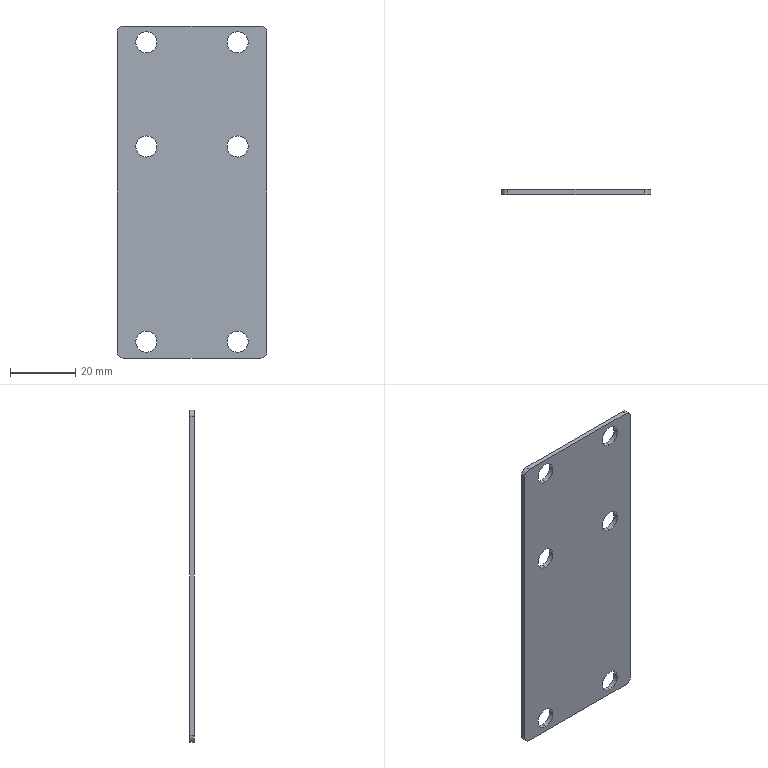Part | SolidWorks | features BaseBody 1 | 1 solid | 22 faces | box 46 x 1.5 x 102 mm | volume 6734 mm3 | cylinder 16 | plane 6 | commonest cylinder face diameters 6.5 x12 4 x4
STEP:
#1=CARTESIAN_POINT('',(14.,0.,-42.75));
#2=VERTEX_POINT('',#1);
#3=CARTESIAN_POINT('',(14.,0.,-49.25));
#4=VERTEX_POINT('',#3);
#5=CARTESIAN_POINT('',(14.,0.,-46.));
#6=DIRECTION('',(0.,1.,0.));
#7=DIRECTION('',(0.,0.,1.));
#8=AXIS2_PLACEMENT_3D('',#5,#6,#7);
#9=CIRCLE('',#8,3.25);
#10=EDGE_CURVE('',#2,#4,#9,.T.);
#11=ORIENTED_EDGE('',*,*,#10,.T.);
#12=CARTESIAN_POINT('',(14.,0.,-46.));
#13=DIRECTION('',(0.,1.,0.));
#14=DIRECTION('',(0.,0.,1.));
#15=AXIS2_PLACEMENT_3D('',#12,#13,#14);
#16=CIRCLE('',#15,3.25);
#17=EDGE_CURVE('',#4,#2,#16,.T.);
#18=ORIENTED_EDGE('',*,*,#17,.T.);
#19=EDGE_LOOP('',(#11,#18));
#20=FACE_BOUND('',#19,.T.);
#21=CARTESIAN_POINT('',(-14.,0.,-42.75));
#22=VERTEX_POINT('',#21);
#23=CARTESIAN_POINT('',(-14.,0.,-49.25));
#24=VERTEX_POINT('',#23);
#25=CARTESIAN_POINT('',(-14.,0.,-46.));
#26=DIRECTION('',(0.,1.,0.));
#27=DIRECTION('',(0.,0.,1.));
#28=AXIS2_PLACEMENT_3D('',#25,#26,#27);
#29=CIRCLE('',#28,3.25);
#30=EDGE_CURVE('',#22,#24,#29,.T.);
#31=ORIENTED_EDGE('',*,*,#30,.T.);
#32=CARTESIAN_POINT('',(-14.,0.,-46.));
#33=DIRECTION('',(0.,1.,0.));
#34=DIRECTION('',(0.,0.,1.));
#35=AXIS2_PLACEMENT_3D('',#32,#33,#34);
#36=CIRCLE('',#35,3.25);
#37=EDGE_CURVE('',#24,#22,#36,.T.);
#38=ORIENTED_EDGE('',*,*,#37,.T.);
#39=EDGE_LOOP('',(#31,#38));
#40=FACE_BOUND('',#39,.T.);
#41=CARTESIAN_POINT('',(-14.,0.,17.25));
#42=VERTEX_POINT('',#41);
#43=CARTESIAN_POINT('',(-14.,0.,10.75));
#44=VERTEX_POINT('',#43);
#45=CARTESIAN_POINT('',(-14.,0.,14.));
#46=DIRECTION('',(0.,1.,0.));
#47=DIRECTION('',(0.,0.,1.));
#48=AXIS2_PLACEMENT_3D('',#45,#46,#47);
#49=CIRCLE('',#48,3.25);
#50=EDGE_CURVE('',#42,#44,#49,.T.);
#51=ORIENTED_EDGE('',*,*,#50,.T.);
#52=CARTESIAN_POINT('',(-14.,0.,14.));
#53=DIRECTION('',(0.,1.,0.));
#54=DIRECTION('',(0.,0.,1.));
#55=AXIS2_PLACEMENT_3D('',#52,#53,#54);
#56=CIRCLE('',#55,3.25);
#57=EDGE_CURVE('',#44,#42,#56,.T.);
#58=ORIENTED_EDGE('',*,*,#57,.T.);
#59=EDGE_LOOP('',(#51,#58));
#60=FACE_BOUND('',#59,.T.);
#61=CARTESIAN_POINT('',(14.,0.,17.25));
#62=VERTEX_POINT('',#61);
#63=CARTESIAN_POINT('',(14.,0.,10.75));
#64=VERTEX_POINT('',#63);
#65=CARTESIAN_POINT('',(14.,0.,14.));
#66=DIRECTION('',(0.,1.,0.));
#67=DIRECTION('',(0.,0.,1.));
#68=AXIS2_PLACEMENT_3D('',#65,#66,#67);
#69=CIRCLE('',#68,3.25);
#70=EDGE_CURVE('',#62,#64,#69,.T.);
#71=ORIENTED_EDGE('',*,*,#70,.T.);
#72=CARTESIAN_POINT('',(14.,0.,14.));
#73=DIRECTION('',(0.,1.,0.));
#74=DIRECTION('',(0.,0.,1.));
#75=AXIS2_PLACEMENT_3D('',#72,#73,#74);
#76=CIRCLE('',#75,3.25);
#77=EDGE_CURVE('',#64,#62,#76,.T.);
#78=ORIENTED_EDGE('',*,*,#77,.T.);
#79=EDGE_LOOP('',(#71,#78));
#80=FACE_BOUND('',#79,.T.);
#81=CARTESIAN_POINT('',(-14.,0.,49.25));
#82=VERTEX_POINT('',#81);
#83=CARTESIAN_POINT('',(-14.,0.,42.75));
#84=VERTEX_POINT('',#83);
#85=CARTESIAN_POINT('',(-14.,0.,46.));
#86=DIRECTION('',(0.,1.,0.));
#87=DIRECTION('',(0.,0.,1.));
#88=AXIS2_PLACEMENT_3D('',#85,#86,#87);
#89=CIRCLE('',#88,3.25);
#90=EDGE_CURVE('',#82,#84,#89,.T.);
#91=ORIENTED_EDGE('',*,*,#90,.T.);
#92=CARTESIAN_POINT('',(-14.,0.,46.));
#93=DIRECTION('',(0.,1.,0.));
#94=DIRECTION('',(0.,0.,1.));
#95=AXIS2_PLACEMENT_3D('',#92,#93,#94);
#96=CIRCLE('',#95,3.25);
#97=EDGE_CURVE('',#84,#82,#96,.T.);
#98=ORIENTED_EDGE('',*,*,#97,.T.);
#99=EDGE_LOOP('',(#91,#98));
#100=FACE_BOUND('',#99,.T.);
#101=CARTESIAN_POINT('',(14.,0.,49.25));
#102=VERTEX_POINT('',#101);
#103=CARTESIAN_POINT('',(14.,0.,42.75));
#104=VERTEX_POINT('',#103);
#105=CARTESIAN_POINT('',(14.,0.,46.));
#106=DIRECTION('',(0.,1.,0.));
#107=DIRECTION('',(0.,0.,1.));
#108=AXIS2_PLACEMENT_3D('',#105,#106,#107);
#109=CIRCLE('',#108,3.25);
#110=EDGE_CURVE('',#102,#104,#109,.T.);
#111=ORIENTED_EDGE('',*,*,#110,.T.);
#112=CARTESIAN_POINT('',(14.,0.,46.));
#113=DIRECTION('',(0.,1.,0.));
#114=DIRECTION('',(0.,0.,1.));
#115=AXIS2_PLACEMENT_3D('',#112,#113,#114);
#116=CIRCLE('',#115,3.25);
#117=EDGE_CURVE('',#104,#102,#116,.T.);
#118=ORIENTED_EDGE('',*,*,#117,.T.);
#119=EDGE_LOOP('',(#111,#118));
#120=FACE_BOUND('',#119,.T.);
#121=CARTESIAN_POINT('',(-23.,0.,49.));
#122=VERTEX_POINT('',#121);
#123=CARTESIAN_POINT('',(-23.,0.,-49.));
#124=VERTEX_POINT('',#123);
#125=CARTESIAN_POINT('',(-23.,0.,-51.));
#126=DIRECTION('',(0.,0.,-1.));
#127=VECTOR('',#126,1000.);
#128=LINE('',#125,#127);
#129=EDGE_CURVE('',#122,#124,#128,.T.);
#130=ORIENTED_EDGE('',*,*,#129,.T.);
#131=CARTESIAN_POINT('',(-21.,0.,-51.));
#132=VERTEX_POINT('',#131);
#133=CARTESIAN_POINT('',(-21.,0.,-49.));
#134=DIRECTION('',(0.,1.,0.));
#135=DIRECTION('',(0.,0.,-1.));
#136=AXIS2_PLACEMENT_3D('',#133,#134,#135);
#137=CIRCLE('',#136,2.);
#138=EDGE_CURVE('',#132,#124,#137,.T.);
#139=ORIENTED_EDGE('',*,*,#138,.F.);
#140=CARTESIAN_POINT('',(21.,0.,-51.));
#141=VERTEX_POINT('',#140);
#142=CARTESIAN_POINT('',(-23.,0.,-51.));
#143=DIRECTION('',(1.,0.,0.));
#144=VECTOR('',#143,1000.);
#145=LINE('',#142,#144);
#146=EDGE_CURVE('',#132,#141,#145,.T.);
#147=ORIENTED_EDGE('',*,*,#146,.T.);
#148=CARTESIAN_POINT('',(23.,0.,-49.));
#149=VERTEX_POINT('',#148);
#150=CARTESIAN_POINT('',(21.,0.,-49.));
#151=DIRECTION('',(0.,1.,0.));
#152=DIRECTION('',(0.,0.,-1.));
#153=AXIS2_PLACEMENT_3D('',#150,#151,#152);
#154=CIRCLE('',#153,2.);
#155=EDGE_CURVE('',#149,#141,#154,.T.);
#156=ORIENTED_EDGE('',*,*,#155,.F.);
#157=CARTESIAN_POINT('',(23.,0.,49.));
#158=VERTEX_POINT('',#157);
#159=CARTESIAN_POINT('',(23.,0.,-51.));
#160=DIRECTION('',(0.,0.,1.));
#161=VECTOR('',#160,1000.);
#162=LINE('',#159,#161);
#163=EDGE_CURVE('',#149,#158,#162,.T.);
#164=ORIENTED_EDGE('',*,*,#163,.T.);
#165=CARTESIAN_POINT('',(21.,0.,51.));
#166=VERTEX_POINT('',#165);
#167=CARTESIAN_POINT('',(21.,0.,49.));
#168=DIRECTION('',(0.,1.,0.));
#169=DIRECTION('',(0.,0.,-1.));
#170=AXIS2_PLACEMENT_3D('',#167,#168,#169);
#171=CIRCLE('',#170,2.);
#172=EDGE_CURVE('',#166,#158,#171,.T.);
#173=ORIENTED_EDGE('',*,*,#172,.F.);
#174=CARTESIAN_POINT('',(-21.,0.,51.));
#175=VERTEX_POINT('',#174);
#176=CARTESIAN_POINT('',(-23.,0.,51.));
#177=DIRECTION('',(-1.,0.,0.));
#178=VECTOR('',#177,1000.);
#179=LINE('',#176,#178);
#180=EDGE_CURVE('',#166,#175,#179,.T.);
#181=ORIENTED_EDGE('',*,*,#180,.T.);
#182=CARTESIAN_POINT('',(-21.,0.,49.));
#183=DIRECTION('',(0.,1.,0.));
#184=DIRECTION('',(0.,0.,-1.));
#185=AXIS2_PLACEMENT_3D('',#182,#183,#184);
#186=CIRCLE('',#185,2.);
#187=EDGE_CURVE('',#122,#175,#186,.T.);
#188=ORIENTED_EDGE('',*,*,#187,.F.);
#189=EDGE_LOOP('',(#130,#139,#147,#156,#164,#173,#181,#188));
#190=FACE_OUTER_BOUND('',#189,.T.);
#191=CARTESIAN_POINT('',(0.,0.,0.));
#192=DIRECTION('',(0.,1.,0.));
#193=DIRECTION('',(1.,0.,0.));
#194=AXIS2_PLACEMENT_3D('',#191,#192,#193);
#195=PLANE('',#194);
#196=ADVANCED_FACE('',(#20,#40,#60,#80,#100,#120,#190),#195,.F.);
#197=ORIENTED_EDGE('',*,*,#146,.F.);
#198=CARTESIAN_POINT('',(-21.,1.5,-51.));
#199=VERTEX_POINT('',#198);
#200=CARTESIAN_POINT('',(-21.,1.5,-51.));
#201=DIRECTION('',(0.,-1.,0.));
#202=VECTOR('',#201,1000.);
#203=LINE('',#200,#202);
#204=EDGE_CURVE('',#199,#132,#203,.T.);
#205=ORIENTED_EDGE('',*,*,#204,.F.);
#206=CARTESIAN_POINT('',(21.,1.5,-51.));
#207=VERTEX_POINT('',#206);
#208=CARTESIAN_POINT('',(0.,1.5,-51.));
#209=DIRECTION('',(-1.,0.,0.));
#210=VECTOR('',#209,1000.);
#211=LINE('',#208,#210);
#212=EDGE_CURVE('',#207,#199,#211,.T.);
#213=ORIENTED_EDGE('',*,*,#212,.F.);
#214=CARTESIAN_POINT('',(21.,1.5,-51.));
#215=DIRECTION('',(0.,1.,0.));
#216=VECTOR('',#215,1000.);
#217=LINE('',#214,#216);
#218=EDGE_CURVE('',#141,#207,#217,.T.);
#219=ORIENTED_EDGE('',*,*,#218,.F.);
#220=EDGE_LOOP('',(#197,#205,#213,#219));
#221=FACE_OUTER_BOUND('',#220,.T.);
#222=CARTESIAN_POINT('',(-23.,1.5,-51.));
#223=DIRECTION('',(0.,0.,1.));
#224=DIRECTION('',(1.,0.,0.));
#225=AXIS2_PLACEMENT_3D('',#222,#223,#224);
#226=PLANE('',#225);
#227=ADVANCED_FACE('',(#221),#226,.F.);
#228=CARTESIAN_POINT('',(-23.,1.5,-49.));
#229=VERTEX_POINT('',#228);
#230=CARTESIAN_POINT('',(-21.,1.5,-49.));
#231=DIRECTION('',(0.,1.,0.));
#232=DIRECTION('',(0.,0.,-1.));
#233=AXIS2_PLACEMENT_3D('',#230,#231,#232);
#234=CIRCLE('',#233,2.);
#235=EDGE_CURVE('',#199,#229,#234,.T.);
#236=ORIENTED_EDGE('',*,*,#235,.F.);
#237=ORIENTED_EDGE('',*,*,#204,.T.);
#238=ORIENTED_EDGE('',*,*,#138,.T.);
#239=CARTESIAN_POINT('',(-23.,1.5,-49.));
#240=DIRECTION('',(0.,1.,0.));
#241=VECTOR('',#240,1000.);
#242=LINE('',#239,#241);
#243=EDGE_CURVE('',#124,#229,#242,.T.);
#244=ORIENTED_EDGE('',*,*,#243,.T.);
#245=EDGE_LOOP('',(#236,#237,#238,#244));
#246=FACE_OUTER_BOUND('',#245,.T.);
#247=CARTESIAN_POINT('',(-21.,1.5,-49.));
#248=DIRECTION('',(0.,-1.,0.));
#249=DIRECTION('',(0.,0.,-1.));
#250=AXIS2_PLACEMENT_3D('',#247,#248,#249);
#251=CYLINDRICAL_SURFACE('',#250,2.);
#252=ADVANCED_FACE('',(#246),#251,.T.);
#253=CARTESIAN_POINT('',(-23.,1.5,49.));
#254=VERTEX_POINT('',#253);
#255=CARTESIAN_POINT('',(-23.,1.5,0.));
#256=DIRECTION('',(0.,0.,1.));
#257=VECTOR('',#256,1000.);
#258=LINE('',#255,#257);
#259=EDGE_CURVE('',#229,#254,#258,.T.);
#260=ORIENTED_EDGE('',*,*,#259,.F.);
#261=ORIENTED_EDGE('',*,*,#243,.F.);
#262=ORIENTED_EDGE('',*,*,#129,.F.);
#263=CARTESIAN_POINT('',(-23.,1.5,49.));
#264=DIRECTION('',(0.,-1.,0.));
#265=VECTOR('',#264,1000.);
#266=LINE('',#263,#265);
#267=EDGE_CURVE('',#254,#122,#266,.T.);
#268=ORIENTED_EDGE('',*,*,#267,.F.);
#269=EDGE_LOOP('',(#260,#261,#262,#268));
#270=FACE_OUTER_BOUND('',#269,.T.);
#271=CARTESIAN_POINT('',(-23.,1.5,-51.));
#272=DIRECTION('',(1.,0.,0.));
#273=DIRECTION('',(0.,0.,-1.));
#274=AXIS2_PLACEMENT_3D('',#271,#272,#273);
#275=PLANE('',#274);
#276=ADVANCED_FACE('',(#270),#275,.F.);
#277=CARTESIAN_POINT('',(-21.,1.5,51.));
#278=VERTEX_POINT('',#277);
#279=CARTESIAN_POINT('',(-21.,1.5,49.));
#280=DIRECTION('',(0.,1.,0.));
#281=DIRECTION('',(0.,0.,-1.));
#282=AXIS2_PLACEMENT_3D('',#279,#280,#281);
#283=CIRCLE('',#282,2.);
#284=EDGE_CURVE('',#254,#278,#283,.T.);
#285=ORIENTED_EDGE('',*,*,#284,.F.);
#286=ORIENTED_EDGE('',*,*,#267,.T.);
#287=ORIENTED_EDGE('',*,*,#187,.T.);
#288=CARTESIAN_POINT('',(-21.,1.5,51.));
#289=DIRECTION('',(0.,1.,0.));
#290=VECTOR('',#289,1000.);
#291=LINE('',#288,#290);
#292=EDGE_CURVE('',#175,#278,#291,.T.);
#293=ORIENTED_EDGE('',*,*,#292,.T.);
#294=EDGE_LOOP('',(#285,#286,#287,#293));
#295=FACE_OUTER_BOUND('',#294,.T.);
#296=CARTESIAN_POINT('',(-21.,1.5,49.));
#297=DIRECTION('',(0.,-1.,0.));
#298=DIRECTION('',(0.,0.,-1.));
#299=AXIS2_PLACEMENT_3D('',#296,#297,#298);
#300=CYLINDRICAL_SURFACE('',#299,2.);
#301=ADVANCED_FACE('',(#295),#300,.T.);
#302=ORIENTED_EDGE('',*,*,#180,.F.);
#303=CARTESIAN_POINT('',(21.,1.5,51.));
#304=VERTEX_POINT('',#303);
#305=CARTESIAN_POINT('',(21.,1.5,51.));
#306=DIRECTION('',(0.,-1.,0.));
#307=VECTOR('',#306,1000.);
#308=LINE('',#305,#307);
#309=EDGE_CURVE('',#304,#166,#308,.T.);
#310=ORIENTED_EDGE('',*,*,#309,.F.);
#311=CARTESIAN_POINT('',(0.,1.5,51.));
#312=DIRECTION('',(1.,0.,0.));
#313=VECTOR('',#312,1000.);
#314=LINE('',#311,#313);
#315=EDGE_CURVE('',#278,#304,#314,.T.);
#316=ORIENTED_EDGE('',*,*,#315,.F.);
#317=ORIENTED_EDGE('',*,*,#292,.F.);
#318=EDGE_LOOP('',(#302,#310,#316,#317));
#319=FACE_OUTER_BOUND('',#318,.T.);
#320=CARTESIAN_POINT('',(-23.,1.5,51.));
#321=DIRECTION('',(0.,0.,-1.));
#322=DIRECTION('',(0.,-1.,0.));
#323=AXIS2_PLACEMENT_3D('',#320,#321,#322);
#324=PLANE('',#323);
#325=ADVANCED_FACE('',(#319),#324,.F.);
#326=CARTESIAN_POINT('',(23.,1.5,49.));
#327=VERTEX_POINT('',#326);
#328=CARTESIAN_POINT('',(21.,1.5,49.));
#329=DIRECTION('',(0.,1.,0.));
#330=DIRECTION('',(0.,0.,-1.));
#331=AXIS2_PLACEMENT_3D('',#328,#329,#330);
#332=CIRCLE('',#331,2.);
#333=EDGE_CURVE('',#304,#327,#332,.T.);
#334=ORIENTED_EDGE('',*,*,#333,.F.);
#335=ORIENTED_EDGE('',*,*,#309,.T.);
#336=ORIENTED_EDGE('',*,*,#172,.T.);
#337=CARTESIAN_POINT('',(23.,1.5,49.));
#338=DIRECTION('',(0.,1.,0.));
#339=VECTOR('',#338,1000.);
#340=LINE('',#337,#339);
#341=EDGE_CURVE('',#158,#327,#340,.T.);
#342=ORIENTED_EDGE('',*,*,#341,.T.);
#343=EDGE_LOOP('',(#334,#335,#336,#342));
#344=FACE_OUTER_BOUND('',#343,.T.);
#345=CARTESIAN_POINT('',(21.,1.5,49.));
#346=DIRECTION('',(0.,-1.,0.));
#347=DIRECTION('',(0.,0.,-1.));
#348=AXIS2_PLACEMENT_3D('',#345,#346,#347);
#349=CYLINDRICAL_SURFACE('',#348,2.);
#350=ADVANCED_FACE('',(#344),#349,.T.);
#351=ORIENTED_EDGE('',*,*,#163,.F.);
#352=CARTESIAN_POINT('',(23.,1.5,-49.));
#353=VERTEX_POINT('',#352);
#354=CARTESIAN_POINT('',(23.,1.5,-49.));
#355=DIRECTION('',(0.,-1.,0.));
#356=VECTOR('',#355,1000.);
#357=LINE('',#354,#356);
#358=EDGE_CURVE('',#353,#149,#357,.T.);
#359=ORIENTED_EDGE('',*,*,#358,.F.);
#360=CARTESIAN_POINT('',(23.,1.5,0.));
#361=DIRECTION('',(0.,0.,-1.));
#362=VECTOR('',#361,1000.);
#363=LINE('',#360,#362);
#364=EDGE_CURVE('',#327,#353,#363,.T.);
#365=ORIENTED_EDGE('',*,*,#364,.F.);
#366=ORIENTED_EDGE('',*,*,#341,.F.);
#367=EDGE_LOOP('',(#351,#359,#365,#366));
#368=FACE_OUTER_BOUND('',#367,.T.);
#369=CARTESIAN_POINT('',(23.,1.5,-51.));
#370=DIRECTION('',(-1.,0.,0.));
#371=DIRECTION('',(0.,1.,0.));
#372=AXIS2_PLACEMENT_3D('',#369,#370,#371);
#373=PLANE('',#372);
#374=ADVANCED_FACE('',(#368),#373,.F.);
#375=CARTESIAN_POINT('',(21.,1.5,-49.));
#376=DIRECTION('',(0.,1.,0.));
#377=DIRECTION('',(0.,0.,-1.));
#378=AXIS2_PLACEMENT_3D('',#375,#376,#377);
#379=CIRCLE('',#378,2.);
#380=EDGE_CURVE('',#353,#207,#379,.T.);
#381=ORIENTED_EDGE('',*,*,#380,.F.);
#382=ORIENTED_EDGE('',*,*,#358,.T.);
#383=ORIENTED_EDGE('',*,*,#155,.T.);
#384=ORIENTED_EDGE('',*,*,#218,.T.);
#385=EDGE_LOOP('',(#381,#382,#383,#384));
#386=FACE_OUTER_BOUND('',#385,.T.);
#387=CARTESIAN_POINT('',(21.,1.5,-49.));
#388=DIRECTION('',(0.,-1.,0.));
#389=DIRECTION('',(0.,0.,-1.));
#390=AXIS2_PLACEMENT_3D('',#387,#388,#389);
#391=CYLINDRICAL_SURFACE('',#390,2.);
#392=ADVANCED_FACE('',(#386),#391,.T.);
#393=CARTESIAN_POINT('',(14.,1.5,-49.25));
#394=VERTEX_POINT('',#393);
#395=CARTESIAN_POINT('',(14.,1.5,-49.25));
#396=DIRECTION('',(0.,1.,0.));
#397=VECTOR('',#396,1000.);
#398=LINE('',#395,#397);
#399=EDGE_CURVE('',#4,#394,#398,.T.);
#400=ORIENTED_EDGE('',*,*,#399,.F.);
#401=ORIENTED_EDGE('',*,*,#10,.F.);
#402=CARTESIAN_POINT('',(14.,1.5,-42.75));
#403=VERTEX_POINT('',#402);
#404=CARTESIAN_POINT('',(14.,1.5,-42.75));
#405=DIRECTION('',(0.,1.,0.));
#406=VECTOR('',#405,1000.);
#407=LINE('',#404,#406);
#408=EDGE_CURVE('',#2,#403,#407,.T.);
#409=ORIENTED_EDGE('',*,*,#408,.T.);
#410=CARTESIAN_POINT('',(14.,1.5,-46.));
#411=DIRECTION('',(0.,-1.,0.));
#412=DIRECTION('',(0.,0.,1.));
#413=AXIS2_PLACEMENT_3D('',#410,#411,#412);
#414=CIRCLE('',#413,3.25);
#415=EDGE_CURVE('',#394,#403,#414,.T.);
#416=ORIENTED_EDGE('',*,*,#415,.F.);
#417=EDGE_LOOP('',(#400,#401,#409,#416));
#418=FACE_OUTER_BOUND('',#417,.T.);
#419=CARTESIAN_POINT('',(14.,1.5,-46.));
#420=DIRECTION('',(0.,1.,0.));
#421=DIRECTION('',(0.,0.,1.));
#422=AXIS2_PLACEMENT_3D('',#419,#420,#421);
#423=CYLINDRICAL_SURFACE('',#422,3.25);
#424=ADVANCED_FACE('',(#418),#423,.F.);
#425=CARTESIAN_POINT('',(-14.,1.5,-49.25));
#426=VERTEX_POINT('',#425);
#427=CARTESIAN_POINT('',(-14.,1.5,-49.25));
#428=DIRECTION('',(0.,1.,0.));
#429=VECTOR('',#428,1000.);
#430=LINE('',#427,#429);
#431=EDGE_CURVE('',#24,#426,#430,.T.);
#432=ORIENTED_EDGE('',*,*,#431,.F.);
#433=ORIENTED_EDGE('',*,*,#30,.F.);
#434=CARTESIAN_POINT('',(-14.,1.5,-42.75));
#435=VERTEX_POINT('',#434);
#436=CARTESIAN_POINT('',(-14.,1.5,-42.75));
#437=DIRECTION('',(0.,1.,0.));
#438=VECTOR('',#437,1000.);
#439=LINE('',#436,#438);
#440=EDGE_CURVE('',#22,#435,#439,.T.);
#441=ORIENTED_EDGE('',*,*,#440,.T.);
#442=CARTESIAN_POINT('',(-14.,1.5,-46.));
#443=DIRECTION('',(0.,-1.,0.));
#444=DIRECTION('',(0.,0.,1.));
#445=AXIS2_PLACEMENT_3D('',#442,#443,#444);
#446=CIRCLE('',#445,3.25);
#447=EDGE_CURVE('',#426,#435,#446,.T.);
#448=ORIENTED_EDGE('',*,*,#447,.F.);
#449=EDGE_LOOP('',(#432,#433,#441,#448));
#450=FACE_OUTER_BOUND('',#449,.T.);
#451=CARTESIAN_POINT('',(-14.,1.5,-46.));
#452=DIRECTION('',(0.,1.,0.));
#453=DIRECTION('',(0.,0.,1.));
#454=AXIS2_PLACEMENT_3D('',#451,#452,#453);
#455=CYLINDRICAL_SURFACE('',#454,3.25);
#456=ADVANCED_FACE('',(#450),#455,.F.);
#457=CARTESIAN_POINT('',(-14.,1.5,10.75));
#458=VERTEX_POINT('',#457);
#459=CARTESIAN_POINT('',(-14.,1.5,10.75));
#460=DIRECTION('',(0.,1.,0.));
#461=VECTOR('',#460,1000.);
#462=LINE('',#459,#461);
#463=EDGE_CURVE('',#44,#458,#462,.T.);
#464=ORIENTED_EDGE('',*,*,#463,.F.);
#465=ORIENTED_EDGE('',*,*,#50,.F.);
#466=CARTESIAN_POINT('',(-14.,1.5,17.25));
#467=VERTEX_POINT('',#466);
#468=CARTESIAN_POINT('',(-14.,1.5,17.25));
#469=DIRECTION('',(0.,1.,0.));
#470=VECTOR('',#469,1000.);
#471=LINE('',#468,#470);
#472=EDGE_CURVE('',#42,#467,#471,.T.);
#473=ORIENTED_EDGE('',*,*,#472,.T.);
#474=CARTESIAN_POINT('',(-14.,1.5,14.));
#475=DIRECTION('',(0.,-1.,0.));
#476=DIRECTION('',(0.,0.,1.));
#477=AXIS2_PLACEMENT_3D('',#474,#475,#476);
#478=CIRCLE('',#477,3.25);
#479=EDGE_CURVE('',#458,#467,#478,.T.);
#480=ORIENTED_EDGE('',*,*,#479,.F.);
#481=EDGE_LOOP('',(#464,#465,#473,#480));
#482=FACE_OUTER_BOUND('',#481,.T.);
#483=CARTESIAN_POINT('',(-14.,1.5,14.));
#484=DIRECTION('',(0.,1.,0.));
#485=DIRECTION('',(0.,0.,1.));
#486=AXIS2_PLACEMENT_3D('',#483,#484,#485);
#487=CYLINDRICAL_SURFACE('',#486,3.25);
#488=ADVANCED_FACE('',(#482),#487,.F.);
#489=CARTESIAN_POINT('',(14.,1.5,10.75));
#490=VERTEX_POINT('',#489);
#491=CARTESIAN_POINT('',(14.,1.5,10.75));
#492=DIRECTION('',(0.,1.,0.));
#493=VECTOR('',#492,1000.);
#494=LINE('',#491,#493);
#495=EDGE_CURVE('',#64,#490,#494,.T.);
#496=ORIENTED_EDGE('',*,*,#495,.F.);
#497=ORIENTED_EDGE('',*,*,#70,.F.);
#498=CARTESIAN_POINT('',(14.,1.5,17.25));
#499=VERTEX_POINT('',#498);
#500=CARTESIAN_POINT('',(14.,1.5,17.25));
#501=DIRECTION('',(0.,1.,0.));
#502=VECTOR('',#501,1000.);
#503=LINE('',#500,#502);
#504=EDGE_CURVE('',#62,#499,#503,.T.);
#505=ORIENTED_EDGE('',*,*,#504,.T.);
#506=CARTESIAN_POINT('',(14.,1.5,14.));
#507=DIRECTION('',(0.,-1.,0.));
#508=DIRECTION('',(0.,0.,1.));
#509=AXIS2_PLACEMENT_3D('',#506,#507,#508);
#510=CIRCLE('',#509,3.25);
#511=EDGE_CURVE('',#490,#499,#510,.T.);
#512=ORIENTED_EDGE('',*,*,#511,.F.);
#513=EDGE_LOOP('',(#496,#497,#505,#512));
#514=FACE_OUTER_BOUND('',#513,.T.);
#515=CARTESIAN_POINT('',(14.,1.5,14.));
#516=DIRECTION('',(0.,1.,0.));
#517=DIRECTION('',(0.,0.,1.));
#518=AXIS2_PLACEMENT_3D('',#515,#516,#517);
#519=CYLINDRICAL_SURFACE('',#518,3.25);
#520=ADVANCED_FACE('',(#514),#519,.F.);
#521=CARTESIAN_POINT('',(-14.,1.5,42.75));
#522=VERTEX_POINT('',#521);
#523=CARTESIAN_POINT('',(-14.,1.5,42.75));
#524=DIRECTION('',(0.,1.,0.));
#525=VECTOR('',#524,1000.);
#526=LINE('',#523,#525);
#527=EDGE_CURVE('',#84,#522,#526,.T.);
#528=ORIENTED_EDGE('',*,*,#527,.F.);
#529=ORIENTED_EDGE('',*,*,#90,.F.);
#530=CARTESIAN_POINT('',(-14.,1.5,49.25));
#531=VERTEX_POINT('',#530);
#532=CARTESIAN_POINT('',(-14.,1.5,49.25));
#533=DIRECTION('',(0.,1.,0.));
#534=VECTOR('',#533,1000.);
#535=LINE('',#532,#534);
#536=EDGE_CURVE('',#82,#531,#535,.T.);
#537=ORIENTED_EDGE('',*,*,#536,.T.);
#538=CARTESIAN_POINT('',(-14.,1.5,46.));
#539=DIRECTION('',(0.,-1.,0.));
#540=DIRECTION('',(0.,0.,1.));
#541=AXIS2_PLACEMENT_3D('',#538,#539,#540);
#542=CIRCLE('',#541,3.25);
#543=EDGE_CURVE('',#522,#531,#542,.T.);
#544=ORIENTED_EDGE('',*,*,#543,.F.);
#545=EDGE_LOOP('',(#528,#529,#537,#544));
#546=FACE_OUTER_BOUND('',#545,.T.);
#547=CARTESIAN_POINT('',(-14.,1.5,46.));
#548=DIRECTION('',(0.,1.,0.));
#549=DIRECTION('',(0.,0.,1.));
#550=AXIS2_PLACEMENT_3D('',#547,#548,#549);
#551=CYLINDRICAL_SURFACE('',#550,3.25);
#552=ADVANCED_FACE('',(#546),#551,.F.);
#553=CARTESIAN_POINT('',(14.,1.5,42.75));
#554=VERTEX_POINT('',#553);
#555=CARTESIAN_POINT('',(14.,1.5,42.75));
#556=DIRECTION('',(0.,1.,0.));
#557=VECTOR('',#556,1000.);
#558=LINE('',#555,#557);
#559=EDGE_CURVE('',#104,#554,#558,.T.);
#560=ORIENTED_EDGE('',*,*,#559,.F.);
#561=ORIENTED_EDGE('',*,*,#110,.F.);
#562=CARTESIAN_POINT('',(14.,1.5,49.25));
#563=VERTEX_POINT('',#562);
#564=CARTESIAN_POINT('',(14.,1.5,49.25));
#565=DIRECTION('',(0.,1.,0.));
#566=VECTOR('',#565,1000.);
#567=LINE('',#564,#566);
#568=EDGE_CURVE('',#102,#563,#567,.T.);
#569=ORIENTED_EDGE('',*,*,#568,.T.);
#570=CARTESIAN_POINT('',(14.,1.5,46.));
#571=DIRECTION('',(0.,-1.,0.));
#572=DIRECTION('',(0.,0.,1.));
#573=AXIS2_PLACEMENT_3D('',#570,#571,#572);
#574=CIRCLE('',#573,3.25);
#575=EDGE_CURVE('',#554,#563,#574,.T.);
#576=ORIENTED_EDGE('',*,*,#575,.F.);
#577=EDGE_LOOP('',(#560,#561,#569,#576));
#578=FACE_OUTER_BOUND('',#577,.T.);
#579=CARTESIAN_POINT('',(14.,1.5,46.));
#580=DIRECTION('',(0.,1.,0.));
#581=DIRECTION('',(0.,0.,1.));
#582=AXIS2_PLACEMENT_3D('',#579,#580,#581);
#583=CYLINDRICAL_SURFACE('',#582,3.25);
#584=ADVANCED_FACE('',(#578),#583,.F.);
#585=CARTESIAN_POINT('',(14.,1.5,-46.));
#586=DIRECTION('',(0.,-1.,0.));
#587=DIRECTION('',(0.,0.,1.));
#588=AXIS2_PLACEMENT_3D('',#585,#586,#587);
#589=CIRCLE('',#588,3.25);
#590=EDGE_CURVE('',#403,#394,#589,.T.);
#591=ORIENTED_EDGE('',*,*,#590,.T.);
#592=ORIENTED_EDGE('',*,*,#415,.T.);
#593=EDGE_LOOP('',(#591,#592));
#594=FACE_BOUND('',#593,.T.);
#595=CARTESIAN_POINT('',(-14.,1.5,-46.));
#596=DIRECTION('',(0.,-1.,0.));
#597=DIRECTION('',(0.,0.,1.));
#598=AXIS2_PLACEMENT_3D('',#595,#596,#597);
#599=CIRCLE('',#598,3.25);
#600=EDGE_CURVE('',#435,#426,#599,.T.);
#601=ORIENTED_EDGE('',*,*,#600,.T.);
#602=ORIENTED_EDGE('',*,*,#447,.T.);
#603=EDGE_LOOP('',(#601,#602));
#604=FACE_BOUND('',#603,.T.);
#605=CARTESIAN_POINT('',(-14.,1.5,14.));
#606=DIRECTION('',(0.,-1.,0.));
#607=DIRECTION('',(0.,0.,1.));
#608=AXIS2_PLACEMENT_3D('',#605,#606,#607);
#609=CIRCLE('',#608,3.25);
#610=EDGE_CURVE('',#467,#458,#609,.T.);
#611=ORIENTED_EDGE('',*,*,#610,.T.);
#612=ORIENTED_EDGE('',*,*,#479,.T.);
#613=EDGE_LOOP('',(#611,#612));
#614=FACE_BOUND('',#613,.T.);
#615=CARTESIAN_POINT('',(14.,1.5,14.));
#616=DIRECTION('',(0.,-1.,0.));
#617=DIRECTION('',(0.,0.,1.));
#618=AXIS2_PLACEMENT_3D('',#615,#616,#617);
#619=CIRCLE('',#618,3.25);
#620=EDGE_CURVE('',#499,#490,#619,.T.);
#621=ORIENTED_EDGE('',*,*,#620,.T.);
#622=ORIENTED_EDGE('',*,*,#511,.T.);
#623=EDGE_LOOP('',(#621,#622));
#624=FACE_BOUND('',#623,.T.);
#625=CARTESIAN_POINT('',(-14.,1.5,46.));
#626=DIRECTION('',(0.,-1.,0.));
#627=DIRECTION('',(0.,0.,1.));
#628=AXIS2_PLACEMENT_3D('',#625,#626,#627);
#629=CIRCLE('',#628,3.25);
#630=EDGE_CURVE('',#531,#522,#629,.T.);
#631=ORIENTED_EDGE('',*,*,#630,.T.);
#632=ORIENTED_EDGE('',*,*,#543,.T.);
#633=EDGE_LOOP('',(#631,#632));
#634=FACE_BOUND('',#633,.T.);
#635=CARTESIAN_POINT('',(14.,1.5,46.));
#636=DIRECTION('',(0.,-1.,0.));
#637=DIRECTION('',(0.,0.,1.));
#638=AXIS2_PLACEMENT_3D('',#635,#636,#637);
#639=CIRCLE('',#638,3.25);
#640=EDGE_CURVE('',#563,#554,#639,.T.);
#641=ORIENTED_EDGE('',*,*,#640,.T.);
#642=ORIENTED_EDGE('',*,*,#575,.T.);
#643=EDGE_LOOP('',(#641,#642));
#644=FACE_BOUND('',#643,.T.);
#645=ORIENTED_EDGE('',*,*,#364,.T.);
#646=ORIENTED_EDGE('',*,*,#380,.T.);
#647=ORIENTED_EDGE('',*,*,#212,.T.);
#648=ORIENTED_EDGE('',*,*,#235,.T.);
#649=ORIENTED_EDGE('',*,*,#259,.T.);
#650=ORIENTED_EDGE('',*,*,#284,.T.);
#651=ORIENTED_EDGE('',*,*,#315,.T.);
#652=ORIENTED_EDGE('',*,*,#333,.T.);
#653=EDGE_LOOP('',(#645,#646,#647,#648,#649,#650,#651,#652));
#654=FACE_OUTER_BOUND('',#653,.T.);
#655=CARTESIAN_POINT('',(0.,1.5,0.));
#656=DIRECTION('',(0.,1.,0.));
#657=DIRECTION('',(1.,0.,0.));
#658=AXIS2_PLACEMENT_3D('',#655,#656,#657);
#659=PLANE('',#658);
#660=ADVANCED_FACE('',(#594,#604,#614,#624,#634,#644,#654),#659,.T.);
#661=ORIENTED_EDGE('',*,*,#17,.F.);
#662=ORIENTED_EDGE('',*,*,#399,.T.);
#663=ORIENTED_EDGE('',*,*,#590,.F.);
#664=ORIENTED_EDGE('',*,*,#408,.F.);
#665=EDGE_LOOP('',(#661,#662,#663,#664));
#666=FACE_OUTER_BOUND('',#665,.T.);
#667=CARTESIAN_POINT('',(14.,1.5,-46.));
#668=DIRECTION('',(0.,1.,0.));
#669=DIRECTION('',(0.,0.,1.));
#670=AXIS2_PLACEMENT_3D('',#667,#668,#669);
#671=CYLINDRICAL_SURFACE('',#670,3.25);
#672=ADVANCED_FACE('',(#666),#671,.F.);
#673=ORIENTED_EDGE('',*,*,#37,.F.);
#674=ORIENTED_EDGE('',*,*,#431,.T.);
#675=ORIENTED_EDGE('',*,*,#600,.F.);
#676=ORIENTED_EDGE('',*,*,#440,.F.);
#677=EDGE_LOOP('',(#673,#674,#675,#676));
#678=FACE_OUTER_BOUND('',#677,.T.);
#679=CARTESIAN_POINT('',(-14.,1.5,-46.));
#680=DIRECTION('',(0.,1.,0.));
#681=DIRECTION('',(0.,0.,1.));
#682=AXIS2_PLACEMENT_3D('',#679,#680,#681);
#683=CYLINDRICAL_SURFACE('',#682,3.25);
#684=ADVANCED_FACE('',(#678),#683,.F.);
#685=ORIENTED_EDGE('',*,*,#57,.F.);
#686=ORIENTED_EDGE('',*,*,#463,.T.);
#687=ORIENTED_EDGE('',*,*,#610,.F.);
#688=ORIENTED_EDGE('',*,*,#472,.F.);
#689=EDGE_LOOP('',(#685,#686,#687,#688));
#690=FACE_OUTER_BOUND('',#689,.T.);
#691=CARTESIAN_POINT('',(-14.,1.5,14.));
#692=DIRECTION('',(0.,1.,0.));
#693=DIRECTION('',(0.,0.,1.));
#694=AXIS2_PLACEMENT_3D('',#691,#692,#693);
#695=CYLINDRICAL_SURFACE('',#694,3.25);
#696=ADVANCED_FACE('',(#690),#695,.F.);
#697=ORIENTED_EDGE('',*,*,#77,.F.);
#698=ORIENTED_EDGE('',*,*,#495,.T.);
#699=ORIENTED_EDGE('',*,*,#620,.F.);
#700=ORIENTED_EDGE('',*,*,#504,.F.);
#701=EDGE_LOOP('',(#697,#698,#699,#700));
#702=FACE_OUTER_BOUND('',#701,.T.);
#703=CARTESIAN_POINT('',(14.,1.5,14.));
#704=DIRECTION('',(0.,1.,0.));
#705=DIRECTION('',(0.,0.,1.));
#706=AXIS2_PLACEMENT_3D('',#703,#704,#705);
#707=CYLINDRICAL_SURFACE('',#706,3.25);
#708=ADVANCED_FACE('',(#702),#707,.F.);
#709=ORIENTED_EDGE('',*,*,#97,.F.);
#710=ORIENTED_EDGE('',*,*,#527,.T.);
#711=ORIENTED_EDGE('',*,*,#630,.F.);
#712=ORIENTED_EDGE('',*,*,#536,.F.);
#713=EDGE_LOOP('',(#709,#710,#711,#712));
#714=FACE_OUTER_BOUND('',#713,.T.);
#715=CARTESIAN_POINT('',(-14.,1.5,46.));
#716=DIRECTION('',(0.,1.,0.));
#717=DIRECTION('',(0.,0.,1.));
#718=AXIS2_PLACEMENT_3D('',#715,#716,#717);
#719=CYLINDRICAL_SURFACE('',#718,3.25);
#720=ADVANCED_FACE('',(#714),#719,.F.);
#721=ORIENTED_EDGE('',*,*,#117,.F.);
#722=ORIENTED_EDGE('',*,*,#559,.T.);
#723=ORIENTED_EDGE('',*,*,#640,.F.);
#724=ORIENTED_EDGE('',*,*,#568,.F.);
#725=EDGE_LOOP('',(#721,#722,#723,#724));
#726=FACE_OUTER_BOUND('',#725,.T.);
#727=CARTESIAN_POINT('',(14.,1.5,46.));
#728=DIRECTION('',(0.,1.,0.));
#729=DIRECTION('',(0.,0.,1.));
#730=AXIS2_PLACEMENT_3D('',#727,#728,#729);
#731=CYLINDRICAL_SURFACE('',#730,3.25);
#732=ADVANCED_FACE('',(#726),#731,.F.);
#733=CLOSED_SHELL('',(#196,#227,#252,#276,#301,#325,#350,#374,#392,#424,#456,#488,#520,#552,#584,#660,#672,#684,#696,#708,#720,#732));
#734=MANIFOLD_SOLID_BREP('',#733);
#735=CARTESIAN_POINT('',(0.,0.,0.));
#736=DIRECTION('',(0.,0.,1.));
#737=DIRECTION('',(1.,0.,0.));
#738=AXIS2_PLACEMENT_3D('',#735,#736,#737);
#739=(LENGTH_UNIT()NAMED_UNIT(*)SI_UNIT(.MILLI.,.METRE.));
#740=UNCERTAINTY_MEASURE_WITH_UNIT(LENGTH_MEASURE(0.00001),#739,'','');
#741=(NAMED_UNIT(*)PLANE_ANGLE_UNIT()SI_UNIT($,.RADIAN.));
#742=(NAMED_UNIT(*)SI_UNIT($,.STERADIAN.)SOLID_ANGLE_UNIT());
#743=(GEOMETRIC_REPRESENTATION_CONTEXT(3)GLOBAL_UNCERTAINTY_ASSIGNED_CONTEXT((#740))GLOBAL_UNIT_ASSIGNED_CONTEXT((#739,#741,#742))REPRESENTATION_CONTEXT('',''));
#744=ADVANCED_BREP_SHAPE_REPRESENTATION('',(#734,#738),#743);